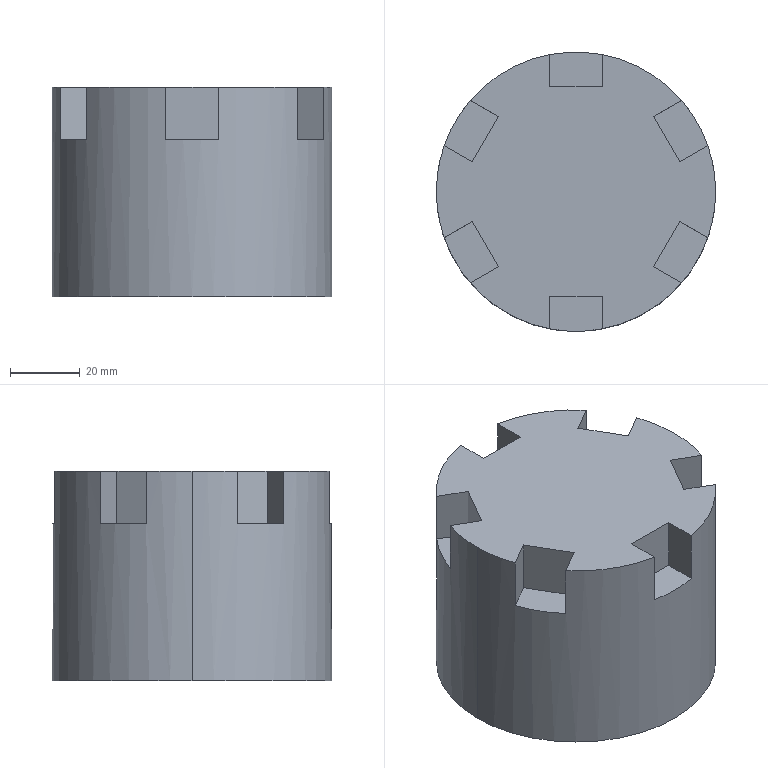Part | SolidWorks | features ICE 3, Extrusion 1 | 1 solid | 35 faces | box 80 x 80 x 60 mm | volume 237992 mm3 | plane 31 | cylinder 4 | commonest cylinder face diameters 39 x2 80 x2
STEP:
#1=CARTESIAN_POINT('',(40.,0.,60.));
#2=VERTEX_POINT('',#1);
#3=CARTESIAN_POINT('',(37.777,13.15,60.));
#4=VERTEX_POINT('',#3);
#5=CARTESIAN_POINT('',(0.,0.,60.));
#6=DIRECTION('',(0.,0.,1.));
#7=DIRECTION('',(1.,0.,0.));
#8=AXIS2_PLACEMENT_3D('',#5,#6,#7);
#9=CIRCLE('',#8,40.);
#10=EDGE_CURVE('',#2,#4,#9,.T.);
#11=ORIENTED_EDGE('',*,*,#10,.F.);
#12=CARTESIAN_POINT('',(40.,0.,0.));
#13=VERTEX_POINT('',#12);
#14=CARTESIAN_POINT('',(40.,0.,60.));
#15=DIRECTION('',(0.,0.,-1.));
#16=VECTOR('',#15,1000.);
#17=LINE('',#14,#16);
#18=EDGE_CURVE('',#2,#13,#17,.T.);
#19=ORIENTED_EDGE('',*,*,#18,.T.);
#20=CARTESIAN_POINT('',(-40.,0.,0.));
#21=VERTEX_POINT('',#20);
#22=CARTESIAN_POINT('',(0.,0.,0.));
#23=DIRECTION('',(0.,0.,1.));
#24=DIRECTION('',(1.,0.,0.));
#25=AXIS2_PLACEMENT_3D('',#22,#23,#24);
#26=CIRCLE('',#25,40.);
#27=EDGE_CURVE('',#13,#21,#26,.T.);
#28=ORIENTED_EDGE('',*,*,#27,.T.);
#29=CARTESIAN_POINT('',(-40.,0.,60.));
#30=VERTEX_POINT('',#29);
#31=CARTESIAN_POINT('',(-40.,0.,60.));
#32=DIRECTION('',(0.,0.,-1.));
#33=VECTOR('',#32,1000.);
#34=LINE('',#31,#33);
#35=EDGE_CURVE('',#30,#21,#34,.T.);
#36=ORIENTED_EDGE('',*,*,#35,.F.);
#37=CARTESIAN_POINT('',(-37.777,13.15,60.));
#38=VERTEX_POINT('',#37);
#39=CARTESIAN_POINT('',(0.,0.,60.));
#40=DIRECTION('',(0.,0.,1.));
#41=DIRECTION('',(1.,0.,0.));
#42=AXIS2_PLACEMENT_3D('',#39,#40,#41);
#43=CIRCLE('',#42,40.);
#44=EDGE_CURVE('',#38,#30,#43,.T.);
#45=ORIENTED_EDGE('',*,*,#44,.F.);
#46=CARTESIAN_POINT('',(-37.777,13.15,45.));
#47=VERTEX_POINT('',#46);
#48=CARTESIAN_POINT('',(-37.777,13.15,45.));
#49=DIRECTION('',(0.,0.,1.));
#50=VECTOR('',#49,1000.);
#51=LINE('',#48,#50);
#52=EDGE_CURVE('',#47,#38,#51,.T.);
#53=ORIENTED_EDGE('',*,*,#52,.F.);
#54=CARTESIAN_POINT('',(-30.277,26.14,45.));
#55=VERTEX_POINT('',#54);
#56=CARTESIAN_POINT('',(0.,0.,45.));
#57=DIRECTION('',(0.,0.,1.));
#58=DIRECTION('',(1.,0.,0.));
#59=AXIS2_PLACEMENT_3D('',#56,#57,#58);
#60=CIRCLE('',#59,40.);
#61=EDGE_CURVE('',#55,#47,#60,.T.);
#62=ORIENTED_EDGE('',*,*,#61,.F.);
#63=CARTESIAN_POINT('',(-30.277,26.14,60.));
#64=VERTEX_POINT('',#63);
#65=CARTESIAN_POINT('',(-30.277,26.14,45.));
#66=DIRECTION('',(0.,0.,1.));
#67=VECTOR('',#66,1000.);
#68=LINE('',#65,#67);
#69=EDGE_CURVE('',#55,#64,#68,.T.);
#70=ORIENTED_EDGE('',*,*,#69,.T.);
#71=CARTESIAN_POINT('',(-7.5,39.291,60.));
#72=VERTEX_POINT('',#71);
#73=CARTESIAN_POINT('',(0.,0.,60.));
#74=DIRECTION('',(0.,0.,1.));
#75=DIRECTION('',(1.,0.,0.));
#76=AXIS2_PLACEMENT_3D('',#73,#74,#75);
#77=CIRCLE('',#76,40.);
#78=EDGE_CURVE('',#72,#64,#77,.T.);
#79=ORIENTED_EDGE('',*,*,#78,.F.);
#80=CARTESIAN_POINT('',(-7.5,39.291,45.));
#81=VERTEX_POINT('',#80);
#82=CARTESIAN_POINT('',(-7.5,39.291,45.));
#83=DIRECTION('',(0.,0.,1.));
#84=VECTOR('',#83,1000.);
#85=LINE('',#82,#84);
#86=EDGE_CURVE('',#81,#72,#85,.T.);
#87=ORIENTED_EDGE('',*,*,#86,.F.);
#88=CARTESIAN_POINT('',(7.5,39.291,45.));
#89=VERTEX_POINT('',#88);
#90=CARTESIAN_POINT('',(0.,0.,45.));
#91=DIRECTION('',(0.,0.,1.));
#92=DIRECTION('',(1.,0.,0.));
#93=AXIS2_PLACEMENT_3D('',#90,#91,#92);
#94=CIRCLE('',#93,40.);
#95=EDGE_CURVE('',#89,#81,#94,.T.);
#96=ORIENTED_EDGE('',*,*,#95,.F.);
#97=CARTESIAN_POINT('',(7.5,39.291,60.));
#98=VERTEX_POINT('',#97);
#99=CARTESIAN_POINT('',(7.5,39.291,45.));
#100=DIRECTION('',(0.,0.,1.));
#101=VECTOR('',#100,1000.);
#102=LINE('',#99,#101);
#103=EDGE_CURVE('',#89,#98,#102,.T.);
#104=ORIENTED_EDGE('',*,*,#103,.T.);
#105=CARTESIAN_POINT('',(30.277,26.14,60.));
#106=VERTEX_POINT('',#105);
#107=CARTESIAN_POINT('',(0.,0.,60.));
#108=DIRECTION('',(0.,0.,1.));
#109=DIRECTION('',(1.,0.,0.));
#110=AXIS2_PLACEMENT_3D('',#107,#108,#109);
#111=CIRCLE('',#110,40.);
#112=EDGE_CURVE('',#106,#98,#111,.T.);
#113=ORIENTED_EDGE('',*,*,#112,.F.);
#114=CARTESIAN_POINT('',(30.277,26.14,45.));
#115=VERTEX_POINT('',#114);
#116=CARTESIAN_POINT('',(30.277,26.14,45.));
#117=DIRECTION('',(0.,0.,1.));
#118=VECTOR('',#117,1000.);
#119=LINE('',#116,#118);
#120=EDGE_CURVE('',#115,#106,#119,.T.);
#121=ORIENTED_EDGE('',*,*,#120,.F.);
#122=CARTESIAN_POINT('',(37.777,13.15,45.));
#123=VERTEX_POINT('',#122);
#124=CARTESIAN_POINT('',(0.,0.,45.));
#125=DIRECTION('',(0.,0.,1.));
#126=DIRECTION('',(1.,0.,0.));
#127=AXIS2_PLACEMENT_3D('',#124,#125,#126);
#128=CIRCLE('',#127,40.);
#129=EDGE_CURVE('',#123,#115,#128,.T.);
#130=ORIENTED_EDGE('',*,*,#129,.F.);
#131=CARTESIAN_POINT('',(37.777,13.15,45.));
#132=DIRECTION('',(0.,0.,1.));
#133=VECTOR('',#132,1000.);
#134=LINE('',#131,#133);
#135=EDGE_CURVE('',#123,#4,#134,.T.);
#136=ORIENTED_EDGE('',*,*,#135,.T.);
#137=EDGE_LOOP('',(#11,#19,#28,#36,#45,#53,#62,#70,#79,#87,#96,#104,#113,#121,#130,#136));
#138=FACE_OUTER_BOUND('',#137,.T.);
#139=CARTESIAN_POINT('',(0.,0.,60.));
#140=DIRECTION('',(0.,0.,-1.));
#141=DIRECTION('',(-1.,0.,0.));
#142=AXIS2_PLACEMENT_3D('',#139,#140,#141);
#143=CYLINDRICAL_SURFACE('',#142,40.);
#144=ADVANCED_FACE('',(#138),#143,.T.);
#145=CARTESIAN_POINT('',(-19.5,0.,40.));
#146=VERTEX_POINT('',#145);
#147=CARTESIAN_POINT('',(19.5,0.,40.));
#148=VERTEX_POINT('',#147);
#149=CARTESIAN_POINT('',(0.,0.,40.));
#150=DIRECTION('',(0.,0.,1.));
#151=DIRECTION('',(1.,0.,0.));
#152=AXIS2_PLACEMENT_3D('',#149,#150,#151);
#153=CIRCLE('',#152,19.5);
#154=EDGE_CURVE('',#146,#148,#153,.T.);
#155=ORIENTED_EDGE('',*,*,#154,.T.);
#156=CARTESIAN_POINT('',(19.5,0.,0.));
#157=VERTEX_POINT('',#156);
#158=CARTESIAN_POINT('',(19.5,0.,40.));
#159=DIRECTION('',(0.,0.,-1.));
#160=VECTOR('',#159,1000.);
#161=LINE('',#158,#160);
#162=EDGE_CURVE('',#148,#157,#161,.T.);
#163=ORIENTED_EDGE('',*,*,#162,.T.);
#164=CARTESIAN_POINT('',(-19.5,0.,0.));
#165=VERTEX_POINT('',#164);
#166=CARTESIAN_POINT('',(0.,0.,0.));
#167=DIRECTION('',(0.,0.,1.));
#168=DIRECTION('',(1.,0.,0.));
#169=AXIS2_PLACEMENT_3D('',#166,#167,#168);
#170=CIRCLE('',#169,19.5);
#171=EDGE_CURVE('',#165,#157,#170,.T.);
#172=ORIENTED_EDGE('',*,*,#171,.F.);
#173=CARTESIAN_POINT('',(-19.5,0.,40.));
#174=DIRECTION('',(0.,0.,-1.));
#175=VECTOR('',#174,1000.);
#176=LINE('',#173,#175);
#177=EDGE_CURVE('',#146,#165,#176,.T.);
#178=ORIENTED_EDGE('',*,*,#177,.F.);
#179=EDGE_LOOP('',(#155,#163,#172,#178));
#180=FACE_OUTER_BOUND('',#179,.T.);
#181=CARTESIAN_POINT('',(0.,0.,40.));
#182=DIRECTION('',(0.,0.,-1.));
#183=DIRECTION('',(-1.,0.,0.));
#184=AXIS2_PLACEMENT_3D('',#181,#182,#183);
#185=CYLINDRICAL_SURFACE('',#184,19.5);
#186=ADVANCED_FACE('',(#180),#185,.F.);
#187=CARTESIAN_POINT('',(0.,0.,0.));
#188=DIRECTION('',(0.,0.,1.));
#189=DIRECTION('',(1.,0.,0.));
#190=AXIS2_PLACEMENT_3D('',#187,#188,#189);
#191=CIRCLE('',#190,40.);
#192=EDGE_CURVE('',#21,#13,#191,.T.);
#193=ORIENTED_EDGE('',*,*,#192,.F.);
#194=ORIENTED_EDGE('',*,*,#27,.F.);
#195=EDGE_LOOP('',(#193,#194));
#196=FACE_OUTER_BOUND('',#195,.T.);
#197=CARTESIAN_POINT('',(-10.,23.,0.));
#198=VERTEX_POINT('',#197);
#199=CARTESIAN_POINT('',(-10.,16.741,0.));
#200=VERTEX_POINT('',#199);
#201=CARTESIAN_POINT('',(-10.,23.,0.));
#202=DIRECTION('',(0.,-1.,0.));
#203=VECTOR('',#202,1000.);
#204=LINE('',#201,#203);
#205=EDGE_CURVE('',#198,#200,#204,.T.);
#206=ORIENTED_EDGE('',*,*,#205,.T.);
#207=CARTESIAN_POINT('',(0.,0.,0.));
#208=DIRECTION('',(0.,0.,1.));
#209=DIRECTION('',(1.,0.,0.));
#210=AXIS2_PLACEMENT_3D('',#207,#208,#209);
#211=CIRCLE('',#210,19.5);
#212=EDGE_CURVE('',#200,#165,#211,.T.);
#213=ORIENTED_EDGE('',*,*,#212,.T.);
#214=ORIENTED_EDGE('',*,*,#171,.T.);
#215=CARTESIAN_POINT('',(10.,16.741,0.));
#216=VERTEX_POINT('',#215);
#217=CARTESIAN_POINT('',(0.,0.,0.));
#218=DIRECTION('',(0.,0.,1.));
#219=DIRECTION('',(1.,0.,0.));
#220=AXIS2_PLACEMENT_3D('',#217,#218,#219);
#221=CIRCLE('',#220,19.5);
#222=EDGE_CURVE('',#157,#216,#221,.T.);
#223=ORIENTED_EDGE('',*,*,#222,.T.);
#224=CARTESIAN_POINT('',(10.,23.,0.));
#225=VERTEX_POINT('',#224);
#226=CARTESIAN_POINT('',(10.,23.,0.));
#227=DIRECTION('',(0.,-1.,0.));
#228=VECTOR('',#227,1000.);
#229=LINE('',#226,#228);
#230=EDGE_CURVE('',#225,#216,#229,.T.);
#231=ORIENTED_EDGE('',*,*,#230,.F.);
#232=CARTESIAN_POINT('',(10.,23.,0.));
#233=DIRECTION('',(-1.,0.,0.));
#234=VECTOR('',#233,1000.);
#235=LINE('',#232,#234);
#236=EDGE_CURVE('',#225,#198,#235,.T.);
#237=ORIENTED_EDGE('',*,*,#236,.T.);
#238=EDGE_LOOP('',(#206,#213,#214,#223,#231,#237));
#239=FACE_BOUND('',#238,.T.);
#240=CARTESIAN_POINT('',(0.,0.,0.));
#241=DIRECTION('',(0.,0.,1.));
#242=DIRECTION('',(1.,0.,0.));
#243=AXIS2_PLACEMENT_3D('',#240,#241,#242);
#244=PLANE('',#243);
#245=ADVANCED_FACE('',(#196,#239),#244,.F.);
#246=ORIENTED_EDGE('',*,*,#162,.F.);
#247=CARTESIAN_POINT('',(0.,0.,40.));
#248=DIRECTION('',(0.,0.,1.));
#249=DIRECTION('',(1.,0.,0.));
#250=AXIS2_PLACEMENT_3D('',#247,#248,#249);
#251=CIRCLE('',#250,19.5);
#252=EDGE_CURVE('',#148,#146,#251,.T.);
#253=ORIENTED_EDGE('',*,*,#252,.T.);
#254=ORIENTED_EDGE('',*,*,#177,.T.);
#255=ORIENTED_EDGE('',*,*,#212,.F.);
#256=CARTESIAN_POINT('',(-10.,16.741,30.));
#257=VERTEX_POINT('',#256);
#258=CARTESIAN_POINT('',(-10.,16.741,40.));
#259=DIRECTION('',(0.,0.,1.));
#260=VECTOR('',#259,1000.);
#261=LINE('',#258,#260);
#262=EDGE_CURVE('',#200,#257,#261,.T.);
#263=ORIENTED_EDGE('',*,*,#262,.T.);
#264=CARTESIAN_POINT('',(10.,16.741,30.));
#265=VERTEX_POINT('',#264);
#266=CARTESIAN_POINT('',(0.,0.,30.));
#267=DIRECTION('',(0.,0.,1.));
#268=DIRECTION('',(1.,0.,0.));
#269=AXIS2_PLACEMENT_3D('',#266,#267,#268);
#270=CIRCLE('',#269,19.5);
#271=EDGE_CURVE('',#265,#257,#270,.T.);
#272=ORIENTED_EDGE('',*,*,#271,.F.);
#273=CARTESIAN_POINT('',(10.,16.741,40.));
#274=DIRECTION('',(0.,0.,1.));
#275=VECTOR('',#274,1000.);
#276=LINE('',#273,#275);
#277=EDGE_CURVE('',#216,#265,#276,.T.);
#278=ORIENTED_EDGE('',*,*,#277,.F.);
#279=ORIENTED_EDGE('',*,*,#222,.F.);
#280=EDGE_LOOP('',(#246,#253,#254,#255,#263,#272,#278,#279));
#281=FACE_OUTER_BOUND('',#280,.T.);
#282=CARTESIAN_POINT('',(0.,0.,40.));
#283=DIRECTION('',(0.,0.,-1.));
#284=DIRECTION('',(-1.,0.,0.));
#285=AXIS2_PLACEMENT_3D('',#282,#283,#284);
#286=CYLINDRICAL_SURFACE('',#285,19.5);
#287=ADVANCED_FACE('',(#281),#286,.F.);
#288=ORIENTED_EDGE('',*,*,#18,.F.);
#289=CARTESIAN_POINT('',(37.777,-13.15,60.));
#290=VERTEX_POINT('',#289);
#291=CARTESIAN_POINT('',(0.,0.,60.));
#292=DIRECTION('',(0.,0.,1.));
#293=DIRECTION('',(1.,0.,0.));
#294=AXIS2_PLACEMENT_3D('',#291,#292,#293);
#295=CIRCLE('',#294,40.);
#296=EDGE_CURVE('',#290,#2,#295,.T.);
#297=ORIENTED_EDGE('',*,*,#296,.F.);
#298=CARTESIAN_POINT('',(37.777,-13.15,45.));
#299=VERTEX_POINT('',#298);
#300=CARTESIAN_POINT('',(37.777,-13.15,45.));
#301=DIRECTION('',(0.,0.,1.));
#302=VECTOR('',#301,1000.);
#303=LINE('',#300,#302);
#304=EDGE_CURVE('',#299,#290,#303,.T.);
#305=ORIENTED_EDGE('',*,*,#304,.F.);
#306=CARTESIAN_POINT('',(30.277,-26.14,45.));
#307=VERTEX_POINT('',#306);
#308=CARTESIAN_POINT('',(0.,0.,45.));
#309=DIRECTION('',(0.,0.,1.));
#310=DIRECTION('',(1.,0.,0.));
#311=AXIS2_PLACEMENT_3D('',#308,#309,#310);
#312=CIRCLE('',#311,40.);
#313=EDGE_CURVE('',#307,#299,#312,.T.);
#314=ORIENTED_EDGE('',*,*,#313,.F.);
#315=CARTESIAN_POINT('',(30.277,-26.14,60.));
#316=VERTEX_POINT('',#315);
#317=CARTESIAN_POINT('',(30.277,-26.14,45.));
#318=DIRECTION('',(0.,0.,1.));
#319=VECTOR('',#318,1000.);
#320=LINE('',#317,#319);
#321=EDGE_CURVE('',#307,#316,#320,.T.);
#322=ORIENTED_EDGE('',*,*,#321,.T.);
#323=CARTESIAN_POINT('',(7.5,-39.291,60.));
#324=VERTEX_POINT('',#323);
#325=CARTESIAN_POINT('',(0.,0.,60.));
#326=DIRECTION('',(0.,0.,1.));
#327=DIRECTION('',(1.,0.,0.));
#328=AXIS2_PLACEMENT_3D('',#325,#326,#327);
#329=CIRCLE('',#328,40.);
#330=EDGE_CURVE('',#324,#316,#329,.T.);
#331=ORIENTED_EDGE('',*,*,#330,.F.);
#332=CARTESIAN_POINT('',(7.5,-39.291,45.));
#333=VERTEX_POINT('',#332);
#334=CARTESIAN_POINT('',(7.5,-39.291,45.));
#335=DIRECTION('',(0.,0.,1.));
#336=VECTOR('',#335,1000.);
#337=LINE('',#334,#336);
#338=EDGE_CURVE('',#333,#324,#337,.T.);
#339=ORIENTED_EDGE('',*,*,#338,.F.);
#340=CARTESIAN_POINT('',(-7.5,-39.291,45.));
#341=VERTEX_POINT('',#340);
#342=CARTESIAN_POINT('',(0.,0.,45.));
#343=DIRECTION('',(0.,0.,1.));
#344=DIRECTION('',(1.,0.,0.));
#345=AXIS2_PLACEMENT_3D('',#342,#343,#344);
#346=CIRCLE('',#345,40.);
#347=EDGE_CURVE('',#341,#333,#346,.T.);
#348=ORIENTED_EDGE('',*,*,#347,.F.);
#349=CARTESIAN_POINT('',(-7.5,-39.291,60.));
#350=VERTEX_POINT('',#349);
#351=CARTESIAN_POINT('',(-7.5,-39.291,45.));
#352=DIRECTION('',(0.,0.,1.));
#353=VECTOR('',#352,1000.);
#354=LINE('',#351,#353);
#355=EDGE_CURVE('',#341,#350,#354,.T.);
#356=ORIENTED_EDGE('',*,*,#355,.T.);
#357=CARTESIAN_POINT('',(-30.277,-26.14,60.));
#358=VERTEX_POINT('',#357);
#359=CARTESIAN_POINT('',(0.,0.,60.));
#360=DIRECTION('',(0.,0.,1.));
#361=DIRECTION('',(1.,0.,0.));
#362=AXIS2_PLACEMENT_3D('',#359,#360,#361);
#363=CIRCLE('',#362,40.);
#364=EDGE_CURVE('',#358,#350,#363,.T.);
#365=ORIENTED_EDGE('',*,*,#364,.F.);
#366=CARTESIAN_POINT('',(-30.277,-26.14,45.));
#367=VERTEX_POINT('',#366);
#368=CARTESIAN_POINT('',(-30.277,-26.14,45.));
#369=DIRECTION('',(0.,0.,1.));
#370=VECTOR('',#369,1000.);
#371=LINE('',#368,#370);
#372=EDGE_CURVE('',#367,#358,#371,.T.);
#373=ORIENTED_EDGE('',*,*,#372,.F.);
#374=CARTESIAN_POINT('',(-37.777,-13.15,45.));
#375=VERTEX_POINT('',#374);
#376=CARTESIAN_POINT('',(0.,0.,45.));
#377=DIRECTION('',(0.,0.,1.));
#378=DIRECTION('',(1.,0.,0.));
#379=AXIS2_PLACEMENT_3D('',#376,#377,#378);
#380=CIRCLE('',#379,40.);
#381=EDGE_CURVE('',#375,#367,#380,.T.);
#382=ORIENTED_EDGE('',*,*,#381,.F.);
#383=CARTESIAN_POINT('',(-37.777,-13.15,60.));
#384=VERTEX_POINT('',#383);
#385=CARTESIAN_POINT('',(-37.777,-13.15,45.));
#386=DIRECTION('',(0.,0.,1.));
#387=VECTOR('',#386,1000.);
#388=LINE('',#385,#387);
#389=EDGE_CURVE('',#375,#384,#388,.T.);
#390=ORIENTED_EDGE('',*,*,#389,.T.);
#391=CARTESIAN_POINT('',(0.,0.,60.));
#392=DIRECTION('',(0.,0.,1.));
#393=DIRECTION('',(1.,0.,0.));
#394=AXIS2_PLACEMENT_3D('',#391,#392,#393);
#395=CIRCLE('',#394,40.);
#396=EDGE_CURVE('',#30,#384,#395,.T.);
#397=ORIENTED_EDGE('',*,*,#396,.F.);
#398=ORIENTED_EDGE('',*,*,#35,.T.);
#399=ORIENTED_EDGE('',*,*,#192,.T.);
#400=EDGE_LOOP('',(#288,#297,#305,#314,#322,#331,#339,#348,#356,#365,#373,#382,#390,#397,#398,#399));
#401=FACE_OUTER_BOUND('',#400,.T.);
#402=CARTESIAN_POINT('',(0.,0.,60.));
#403=DIRECTION('',(0.,0.,-1.));
#404=DIRECTION('',(-1.,0.,0.));
#405=AXIS2_PLACEMENT_3D('',#402,#403,#404);
#406=CYLINDRICAL_SURFACE('',#405,40.);
#407=ADVANCED_FACE('',(#401),#406,.T.);
#408=CARTESIAN_POINT('',(7.5,30.,60.));
#409=VERTEX_POINT('',#408);
#410=CARTESIAN_POINT('',(7.5,39.291,60.));
#411=DIRECTION('',(0.,1.,0.));
#412=VECTOR('',#411,1000.);
#413=LINE('',#410,#412);
#414=EDGE_CURVE('',#409,#98,#413,.T.);
#415=ORIENTED_EDGE('',*,*,#414,.F.);
#416=CARTESIAN_POINT('',(-7.5,30.,60.));
#417=VERTEX_POINT('',#416);
#418=CARTESIAN_POINT('',(-7.5,30.,60.));
#419=DIRECTION('',(1.,0.,0.));
#420=VECTOR('',#419,1000.);
#421=LINE('',#418,#420);
#422=EDGE_CURVE('',#417,#409,#421,.T.);
#423=ORIENTED_EDGE('',*,*,#422,.F.);
#424=CARTESIAN_POINT('',(-7.5,39.291,60.));
#425=DIRECTION('',(0.,-1.,0.));
#426=VECTOR('',#425,1000.);
#427=LINE('',#424,#426);
#428=EDGE_CURVE('',#72,#417,#427,.T.);
#429=ORIENTED_EDGE('',*,*,#428,.F.);
#430=ORIENTED_EDGE('',*,*,#78,.T.);
#431=CARTESIAN_POINT('',(-22.231,21.495,60.));
#432=VERTEX_POINT('',#431);
#433=CARTESIAN_POINT('',(-30.277,26.14,60.));
#434=DIRECTION('',(-0.866,0.5,0.));
#435=VECTOR('',#434,1000.);
#436=LINE('',#433,#435);
#437=EDGE_CURVE('',#432,#64,#436,.T.);
#438=ORIENTED_EDGE('',*,*,#437,.F.);
#439=CARTESIAN_POINT('',(-29.731,8.505,60.));
#440=VERTEX_POINT('',#439);
#441=CARTESIAN_POINT('',(-29.731,8.505,60.));
#442=DIRECTION('',(0.5,0.866,0.));
#443=VECTOR('',#442,1000.);
#444=LINE('',#441,#443);
#445=EDGE_CURVE('',#440,#432,#444,.T.);
#446=ORIENTED_EDGE('',*,*,#445,.F.);
#447=CARTESIAN_POINT('',(-37.777,13.15,60.));
#448=DIRECTION('',(0.866,-0.5,0.));
#449=VECTOR('',#448,1000.);
#450=LINE('',#447,#449);
#451=EDGE_CURVE('',#38,#440,#450,.T.);
#452=ORIENTED_EDGE('',*,*,#451,.F.);
#453=ORIENTED_EDGE('',*,*,#44,.T.);
#454=ORIENTED_EDGE('',*,*,#396,.T.);
#455=CARTESIAN_POINT('',(-29.731,-8.505,60.));
#456=VERTEX_POINT('',#455);
#457=CARTESIAN_POINT('',(-37.777,-13.15,60.));
#458=DIRECTION('',(-0.866,-0.5,0.));
#459=VECTOR('',#458,1000.);
#460=LINE('',#457,#459);
#461=EDGE_CURVE('',#456,#384,#460,.T.);
#462=ORIENTED_EDGE('',*,*,#461,.F.);
#463=CARTESIAN_POINT('',(-22.231,-21.495,60.));
#464=VERTEX_POINT('',#463);
#465=CARTESIAN_POINT('',(-22.231,-21.495,60.));
#466=DIRECTION('',(-0.5,0.866,0.));
#467=VECTOR('',#466,1000.);
#468=LINE('',#465,#467);
#469=EDGE_CURVE('',#464,#456,#468,.T.);
#470=ORIENTED_EDGE('',*,*,#469,.F.);
#471=CARTESIAN_POINT('',(-30.277,-26.14,60.));
#472=DIRECTION('',(0.866,0.5,0.));
#473=VECTOR('',#472,1000.);
#474=LINE('',#471,#473);
#475=EDGE_CURVE('',#358,#464,#474,.T.);
#476=ORIENTED_EDGE('',*,*,#475,.F.);
#477=ORIENTED_EDGE('',*,*,#364,.T.);
#478=CARTESIAN_POINT('',(-7.5,-30.,60.));
#479=VERTEX_POINT('',#478);
#480=CARTESIAN_POINT('',(-7.5,-39.291,60.));
#481=DIRECTION('',(0.,-1.,0.));
#482=VECTOR('',#481,1000.);
#483=LINE('',#480,#482);
#484=EDGE_CURVE('',#479,#350,#483,.T.);
#485=ORIENTED_EDGE('',*,*,#484,.F.);
#486=CARTESIAN_POINT('',(7.5,-30.,60.));
#487=VERTEX_POINT('',#486);
#488=CARTESIAN_POINT('',(7.5,-30.,60.));
#489=DIRECTION('',(-1.,0.,0.));
#490=VECTOR('',#489,1000.);
#491=LINE('',#488,#490);
#492=EDGE_CURVE('',#487,#479,#491,.T.);
#493=ORIENTED_EDGE('',*,*,#492,.F.);
#494=CARTESIAN_POINT('',(7.5,-39.291,60.));
#495=DIRECTION('',(0.,1.,0.));
#496=VECTOR('',#495,1000.);
#497=LINE('',#494,#496);
#498=EDGE_CURVE('',#324,#487,#497,.T.);
#499=ORIENTED_EDGE('',*,*,#498,.F.);
#500=ORIENTED_EDGE('',*,*,#330,.T.);
#501=CARTESIAN_POINT('',(22.231,-21.495,60.));
#502=VERTEX_POINT('',#501);
#503=CARTESIAN_POINT('',(30.277,-26.14,60.));
#504=DIRECTION('',(0.866,-0.5,0.));
#505=VECTOR('',#504,1000.);
#506=LINE('',#503,#505);
#507=EDGE_CURVE('',#502,#316,#506,.T.);
#508=ORIENTED_EDGE('',*,*,#507,.F.);
#509=CARTESIAN_POINT('',(29.731,-8.505,60.));
#510=VERTEX_POINT('',#509);
#511=CARTESIAN_POINT('',(29.731,-8.505,60.));
#512=DIRECTION('',(-0.5,-0.866,0.));
#513=VECTOR('',#512,1000.);
#514=LINE('',#511,#513);
#515=EDGE_CURVE('',#510,#502,#514,.T.);
#516=ORIENTED_EDGE('',*,*,#515,.F.);
#517=CARTESIAN_POINT('',(37.777,-13.15,60.));
#518=DIRECTION('',(-0.866,0.5,0.));
#519=VECTOR('',#518,1000.);
#520=LINE('',#517,#519);
#521=EDGE_CURVE('',#290,#510,#520,.T.);
#522=ORIENTED_EDGE('',*,*,#521,.F.);
#523=ORIENTED_EDGE('',*,*,#296,.T.);
#524=ORIENTED_EDGE('',*,*,#10,.T.);
#525=CARTESIAN_POINT('',(29.731,8.505,60.));
#526=VERTEX_POINT('',#525);
#527=CARTESIAN_POINT('',(37.777,13.15,60.));
#528=DIRECTION('',(0.866,0.5,0.));
#529=VECTOR('',#528,1000.);
#530=LINE('',#527,#529);
#531=EDGE_CURVE('',#526,#4,#530,.T.);
#532=ORIENTED_EDGE('',*,*,#531,.F.);
#533=CARTESIAN_POINT('',(22.231,21.495,60.));
#534=VERTEX_POINT('',#533);
#535=CARTESIAN_POINT('',(22.231,21.495,60.));
#536=DIRECTION('',(0.5,-0.866,0.));
#537=VECTOR('',#536,1000.);
#538=LINE('',#535,#537);
#539=EDGE_CURVE('',#534,#526,#538,.T.);
#540=ORIENTED_EDGE('',*,*,#539,.F.);
#541=CARTESIAN_POINT('',(30.277,26.14,60.));
#542=DIRECTION('',(-0.866,-0.5,0.));
#543=VECTOR('',#542,1000.);
#544=LINE('',#541,#543);
#545=EDGE_CURVE('',#106,#534,#544,.T.);
#546=ORIENTED_EDGE('',*,*,#545,.F.);
#547=ORIENTED_EDGE('',*,*,#112,.T.);
#548=EDGE_LOOP('',(#415,#423,#429,#430,#438,#446,#452,#453,#454,#462,#470,#476,#477,#485,#493,#499,#500,#508,#516,#522,#523,#524,#532,#540,#546,#547));
#549=FACE_OUTER_BOUND('',#548,.T.);
#550=CARTESIAN_POINT('',(0.,0.,60.));
#551=DIRECTION('',(0.,0.,1.));
#552=DIRECTION('',(1.,0.,0.));
#553=AXIS2_PLACEMENT_3D('',#550,#551,#552);
#554=PLANE('',#553);
#555=ADVANCED_FACE('',(#549),#554,.T.);
#556=ORIENTED_EDGE('',*,*,#154,.F.);
#557=ORIENTED_EDGE('',*,*,#252,.F.);
#558=EDGE_LOOP('',(#556,#557));
#559=FACE_OUTER_BOUND('',#558,.T.);
#560=CARTESIAN_POINT('',(0.,0.,40.));
#561=DIRECTION('',(0.,0.,1.));
#562=DIRECTION('',(1.,0.,0.));
#563=AXIS2_PLACEMENT_3D('',#560,#561,#562);
#564=PLANE('',#563);
#565=ADVANCED_FACE('',(#559),#564,.F.);
#566=ORIENTED_EDGE('',*,*,#531,.T.);
#567=ORIENTED_EDGE('',*,*,#135,.F.);
#568=CARTESIAN_POINT('',(29.731,8.505,45.));
#569=VERTEX_POINT('',#568);
#570=CARTESIAN_POINT('',(37.777,13.15,45.));
#571=DIRECTION('',(0.866,0.5,0.));
#572=VECTOR('',#571,1000.);
#573=LINE('',#570,#572);
#574=EDGE_CURVE('',#569,#123,#573,.T.);
#575=ORIENTED_EDGE('',*,*,#574,.F.);
#576=CARTESIAN_POINT('',(29.731,8.505,45.));
#577=DIRECTION('',(0.,0.,1.));
#578=VECTOR('',#577,1000.);
#579=LINE('',#576,#578);
#580=EDGE_CURVE('',#569,#526,#579,.T.);
#581=ORIENTED_EDGE('',*,*,#580,.T.);
#582=EDGE_LOOP('',(#566,#567,#575,#581));
#583=FACE_OUTER_BOUND('',#582,.T.);
#584=CARTESIAN_POINT('',(37.777,13.15,45.));
#585=DIRECTION('',(0.5,-0.866,0.));
#586=DIRECTION('',(0.866,0.5,0.));
#587=AXIS2_PLACEMENT_3D('',#584,#585,#586);
#588=PLANE('',#587);
#589=ADVANCED_FACE('',(#583),#588,.F.);
#590=ORIENTED_EDGE('',*,*,#539,.T.);
#591=ORIENTED_EDGE('',*,*,#580,.F.);
#592=CARTESIAN_POINT('',(22.231,21.495,45.));
#593=VERTEX_POINT('',#592);
#594=CARTESIAN_POINT('',(22.231,21.495,45.));
#595=DIRECTION('',(0.5,-0.866,0.));
#596=VECTOR('',#595,1000.);
#597=LINE('',#594,#596);
#598=EDGE_CURVE('',#593,#569,#597,.T.);
#599=ORIENTED_EDGE('',*,*,#598,.F.);
#600=CARTESIAN_POINT('',(22.231,21.495,45.));
#601=DIRECTION('',(0.,0.,1.));
#602=VECTOR('',#601,1000.);
#603=LINE('',#600,#602);
#604=EDGE_CURVE('',#593,#534,#603,.T.);
#605=ORIENTED_EDGE('',*,*,#604,.T.);
#606=EDGE_LOOP('',(#590,#591,#599,#605));
#607=FACE_OUTER_BOUND('',#606,.T.);
#608=CARTESIAN_POINT('',(22.231,21.495,45.));
#609=DIRECTION('',(-0.866,-0.5,0.));
#610=DIRECTION('',(0.5,-0.866,0.));
#611=AXIS2_PLACEMENT_3D('',#608,#609,#610);
#612=PLANE('',#611);
#613=ADVANCED_FACE('',(#607),#612,.F.);
#614=ORIENTED_EDGE('',*,*,#545,.T.);
#615=ORIENTED_EDGE('',*,*,#604,.F.);
#616=CARTESIAN_POINT('',(30.277,26.14,45.));
#617=DIRECTION('',(-0.866,-0.5,0.));
#618=VECTOR('',#617,1000.);
#619=LINE('',#616,#618);
#620=EDGE_CURVE('',#115,#593,#619,.T.);
#621=ORIENTED_EDGE('',*,*,#620,.F.);
#622=ORIENTED_EDGE('',*,*,#120,.T.);
#623=EDGE_LOOP('',(#614,#615,#621,#622));
#624=FACE_OUTER_BOUND('',#623,.T.);
#625=CARTESIAN_POINT('',(30.277,26.14,45.));
#626=DIRECTION('',(-0.5,0.866,0.));
#627=DIRECTION('',(-0.866,-0.5,0.));
#628=AXIS2_PLACEMENT_3D('',#625,#626,#627);
#629=PLANE('',#628);
#630=ADVANCED_FACE('',(#624),#629,.F.);
#631=ORIENTED_EDGE('',*,*,#129,.T.);
#632=ORIENTED_EDGE('',*,*,#620,.T.);
#633=ORIENTED_EDGE('',*,*,#598,.T.);
#634=ORIENTED_EDGE('',*,*,#574,.T.);
#635=EDGE_LOOP('',(#631,#632,#633,#634));
#636=FACE_OUTER_BOUND('',#635,.T.);
#637=CARTESIAN_POINT('',(0.,0.,45.));
#638=DIRECTION('',(0.,0.,1.));
#639=DIRECTION('',(1.,0.,0.));
#640=AXIS2_PLACEMENT_3D('',#637,#638,#639);
#641=PLANE('',#640);
#642=ADVANCED_FACE('',(#636),#641,.T.);
#643=ORIENTED_EDGE('',*,*,#507,.T.);
#644=ORIENTED_EDGE('',*,*,#321,.F.);
#645=CARTESIAN_POINT('',(22.231,-21.495,45.));
#646=VERTEX_POINT('',#645);
#647=CARTESIAN_POINT('',(30.277,-26.14,45.));
#648=DIRECTION('',(0.866,-0.5,0.));
#649=VECTOR('',#648,1000.);
#650=LINE('',#647,#649);
#651=EDGE_CURVE('',#646,#307,#650,.T.);
#652=ORIENTED_EDGE('',*,*,#651,.F.);
#653=CARTESIAN_POINT('',(22.231,-21.495,45.));
#654=DIRECTION('',(0.,0.,1.));
#655=VECTOR('',#654,1000.);
#656=LINE('',#653,#655);
#657=EDGE_CURVE('',#646,#502,#656,.T.);
#658=ORIENTED_EDGE('',*,*,#657,.T.);
#659=EDGE_LOOP('',(#643,#644,#652,#658));
#660=FACE_OUTER_BOUND('',#659,.T.);
#661=CARTESIAN_POINT('',(30.277,-26.14,45.));
#662=DIRECTION('',(-0.5,-0.866,0.));
#663=DIRECTION('',(0.866,-0.5,0.));
#664=AXIS2_PLACEMENT_3D('',#661,#662,#663);
#665=PLANE('',#664);
#666=ADVANCED_FACE('',(#660),#665,.F.);
#667=ORIENTED_EDGE('',*,*,#515,.T.);
#668=ORIENTED_EDGE('',*,*,#657,.F.);
#669=CARTESIAN_POINT('',(29.731,-8.505,45.));
#670=VERTEX_POINT('',#669);
#671=CARTESIAN_POINT('',(29.731,-8.505,45.));
#672=DIRECTION('',(-0.5,-0.866,0.));
#673=VECTOR('',#672,1000.);
#674=LINE('',#671,#673);
#675=EDGE_CURVE('',#670,#646,#674,.T.);
#676=ORIENTED_EDGE('',*,*,#675,.F.);
#677=CARTESIAN_POINT('',(29.731,-8.505,45.));
#678=DIRECTION('',(0.,0.,1.));
#679=VECTOR('',#678,1000.);
#680=LINE('',#677,#679);
#681=EDGE_CURVE('',#670,#510,#680,.T.);
#682=ORIENTED_EDGE('',*,*,#681,.T.);
#683=EDGE_LOOP('',(#667,#668,#676,#682));
#684=FACE_OUTER_BOUND('',#683,.T.);
#685=CARTESIAN_POINT('',(29.731,-8.505,45.));
#686=DIRECTION('',(-0.866,0.5,0.));
#687=DIRECTION('',(-0.5,-0.866,0.));
#688=AXIS2_PLACEMENT_3D('',#685,#686,#687);
#689=PLANE('',#688);
#690=ADVANCED_FACE('',(#684),#689,.F.);
#691=ORIENTED_EDGE('',*,*,#521,.T.);
#692=ORIENTED_EDGE('',*,*,#681,.F.);
#693=CARTESIAN_POINT('',(37.777,-13.15,45.));
#694=DIRECTION('',(-0.866,0.5,0.));
#695=VECTOR('',#694,1000.);
#696=LINE('',#693,#695);
#697=EDGE_CURVE('',#299,#670,#696,.T.);
#698=ORIENTED_EDGE('',*,*,#697,.F.);
#699=ORIENTED_EDGE('',*,*,#304,.T.);
#700=EDGE_LOOP('',(#691,#692,#698,#699));
#701=FACE_OUTER_BOUND('',#700,.T.);
#702=CARTESIAN_POINT('',(37.777,-13.15,45.));
#703=DIRECTION('',(0.5,0.866,0.));
#704=DIRECTION('',(-0.866,0.5,0.));
#705=AXIS2_PLACEMENT_3D('',#702,#703,#704);
#706=PLANE('',#705);
#707=ADVANCED_FACE('',(#701),#706,.F.);
#708=ORIENTED_EDGE('',*,*,#313,.T.);
#709=ORIENTED_EDGE('',*,*,#697,.T.);
#710=ORIENTED_EDGE('',*,*,#675,.T.);
#711=ORIENTED_EDGE('',*,*,#651,.T.);
#712=EDGE_LOOP('',(#708,#709,#710,#711));
#713=FACE_OUTER_BOUND('',#712,.T.);
#714=CARTESIAN_POINT('',(0.,0.,45.));
#715=DIRECTION('',(0.,0.,1.));
#716=DIRECTION('',(1.,0.,0.));
#717=AXIS2_PLACEMENT_3D('',#714,#715,#716);
#718=PLANE('',#717);
#719=ADVANCED_FACE('',(#713),#718,.T.);
#720=ORIENTED_EDGE('',*,*,#484,.T.);
#721=ORIENTED_EDGE('',*,*,#355,.F.);
#722=CARTESIAN_POINT('',(-7.5,-30.,45.));
#723=VERTEX_POINT('',#722);
#724=CARTESIAN_POINT('',(-7.5,-39.291,45.));
#725=DIRECTION('',(0.,-1.,0.));
#726=VECTOR('',#725,1000.);
#727=LINE('',#724,#726);
#728=EDGE_CURVE('',#723,#341,#727,.T.);
#729=ORIENTED_EDGE('',*,*,#728,.F.);
#730=CARTESIAN_POINT('',(-7.5,-30.,45.));
#731=DIRECTION('',(0.,0.,1.));
#732=VECTOR('',#731,1000.);
#733=LINE('',#730,#732);
#734=EDGE_CURVE('',#723,#479,#733,.T.);
#735=ORIENTED_EDGE('',*,*,#734,.T.);
#736=EDGE_LOOP('',(#720,#721,#729,#735));
#737=FACE_OUTER_BOUND('',#736,.T.);
#738=CARTESIAN_POINT('',(-7.5,-39.291,45.));
#739=DIRECTION('',(-1.,0.,0.));
#740=DIRECTION('',(0.,-1.,0.));
#741=AXIS2_PLACEMENT_3D('',#738,#739,#740);
#742=PLANE('',#741);
#743=ADVANCED_FACE('',(#737),#742,.F.);
#744=ORIENTED_EDGE('',*,*,#492,.T.);
#745=ORIENTED_EDGE('',*,*,#734,.F.);
#746=CARTESIAN_POINT('',(7.5,-30.,45.));
#747=VERTEX_POINT('',#746);
#748=CARTESIAN_POINT('',(7.5,-30.,45.));
#749=DIRECTION('',(-1.,0.,0.));
#750=VECTOR('',#749,1000.);
#751=LINE('',#748,#750);
#752=EDGE_CURVE('',#747,#723,#751,.T.);
#753=ORIENTED_EDGE('',*,*,#752,.F.);
#754=CARTESIAN_POINT('',(7.5,-30.,45.));
#755=DIRECTION('',(0.,0.,1.));
#756=VECTOR('',#755,1000.);
#757=LINE('',#754,#756);
#758=EDGE_CURVE('',#747,#487,#757,.T.);
#759=ORIENTED_EDGE('',*,*,#758,.T.);
#760=EDGE_LOOP('',(#744,#745,#753,#759));
#761=FACE_OUTER_BOUND('',#760,.T.);
#762=CARTESIAN_POINT('',(7.5,-30.,45.));
#763=DIRECTION('',(0.,1.,0.));
#764=DIRECTION('',(-1.,0.,0.));
#765=AXIS2_PLACEMENT_3D('',#762,#763,#764);
#766=PLANE('',#765);
#767=ADVANCED_FACE('',(#761),#766,.F.);
#768=ORIENTED_EDGE('',*,*,#498,.T.);
#769=ORIENTED_EDGE('',*,*,#758,.F.);
#770=CARTESIAN_POINT('',(7.5,-39.291,45.));
#771=DIRECTION('',(0.,1.,0.));
#772=VECTOR('',#771,1000.);
#773=LINE('',#770,#772);
#774=EDGE_CURVE('',#333,#747,#773,.T.);
#775=ORIENTED_EDGE('',*,*,#774,.F.);
#776=ORIENTED_EDGE('',*,*,#338,.T.);
#777=EDGE_LOOP('',(#768,#769,#775,#776));
#778=FACE_OUTER_BOUND('',#777,.T.);
#779=CARTESIAN_POINT('',(7.5,-39.291,45.));
#780=DIRECTION('',(1.,0.,0.));
#781=DIRECTION('',(0.,1.,0.));
#782=AXIS2_PLACEMENT_3D('',#779,#780,#781);
#783=PLANE('',#782);
#784=ADVANCED_FACE('',(#778),#783,.F.);
#785=ORIENTED_EDGE('',*,*,#347,.T.);
#786=ORIENTED_EDGE('',*,*,#774,.T.);
#787=ORIENTED_EDGE('',*,*,#752,.T.);
#788=ORIENTED_EDGE('',*,*,#728,.T.);
#789=EDGE_LOOP('',(#785,#786,#787,#788));
#790=FACE_OUTER_BOUND('',#789,.T.);
#791=CARTESIAN_POINT('',(0.,0.,45.));
#792=DIRECTION('',(0.,0.,1.));
#793=DIRECTION('',(1.,0.,0.));
#794=AXIS2_PLACEMENT_3D('',#791,#792,#793);
#795=PLANE('',#794);
#796=ADVANCED_FACE('',(#790),#795,.T.);
#797=ORIENTED_EDGE('',*,*,#461,.T.);
#798=ORIENTED_EDGE('',*,*,#389,.F.);
#799=CARTESIAN_POINT('',(-29.731,-8.505,45.));
#800=VERTEX_POINT('',#799);
#801=CARTESIAN_POINT('',(-37.777,-13.15,45.));
#802=DIRECTION('',(-0.866,-0.5,0.));
#803=VECTOR('',#802,1000.);
#804=LINE('',#801,#803);
#805=EDGE_CURVE('',#800,#375,#804,.T.);
#806=ORIENTED_EDGE('',*,*,#805,.F.);
#807=CARTESIAN_POINT('',(-29.731,-8.505,45.));
#808=DIRECTION('',(0.,0.,1.));
#809=VECTOR('',#808,1000.);
#810=LINE('',#807,#809);
#811=EDGE_CURVE('',#800,#456,#810,.T.);
#812=ORIENTED_EDGE('',*,*,#811,.T.);
#813=EDGE_LOOP('',(#797,#798,#806,#812));
#814=FACE_OUTER_BOUND('',#813,.T.);
#815=CARTESIAN_POINT('',(-37.777,-13.15,45.));
#816=DIRECTION('',(-0.5,0.866,0.));
#817=DIRECTION('',(-0.866,-0.5,0.));
#818=AXIS2_PLACEMENT_3D('',#815,#816,#817);
#819=PLANE('',#818);
#820=ADVANCED_FACE('',(#814),#819,.F.);
#821=ORIENTED_EDGE('',*,*,#469,.T.);
#822=ORIENTED_EDGE('',*,*,#811,.F.);
#823=CARTESIAN_POINT('',(-22.231,-21.495,45.));
#824=VERTEX_POINT('',#823);
#825=CARTESIAN_POINT('',(-22.231,-21.495,45.));
#826=DIRECTION('',(-0.5,0.866,0.));
#827=VECTOR('',#826,1000.);
#828=LINE('',#825,#827);
#829=EDGE_CURVE('',#824,#800,#828,.T.);
#830=ORIENTED_EDGE('',*,*,#829,.F.);
#831=CARTESIAN_POINT('',(-22.231,-21.495,45.));
#832=DIRECTION('',(0.,0.,1.));
#833=VECTOR('',#832,1000.);
#834=LINE('',#831,#833);
#835=EDGE_CURVE('',#824,#464,#834,.T.);
#836=ORIENTED_EDGE('',*,*,#835,.T.);
#837=EDGE_LOOP('',(#821,#822,#830,#836));
#838=FACE_OUTER_BOUND('',#837,.T.);
#839=CARTESIAN_POINT('',(-22.231,-21.495,45.));
#840=DIRECTION('',(0.866,0.5,0.));
#841=DIRECTION('',(-0.5,0.866,0.));
#842=AXIS2_PLACEMENT_3D('',#839,#840,#841);
#843=PLANE('',#842);
#844=ADVANCED_FACE('',(#838),#843,.F.);
#845=ORIENTED_EDGE('',*,*,#475,.T.);
#846=ORIENTED_EDGE('',*,*,#835,.F.);
#847=CARTESIAN_POINT('',(-30.277,-26.14,45.));
#848=DIRECTION('',(0.866,0.5,0.));
#849=VECTOR('',#848,1000.);
#850=LINE('',#847,#849);
#851=EDGE_CURVE('',#367,#824,#850,.T.);
#852=ORIENTED_EDGE('',*,*,#851,.F.);
#853=ORIENTED_EDGE('',*,*,#372,.T.);
#854=EDGE_LOOP('',(#845,#846,#852,#853));
#855=FACE_OUTER_BOUND('',#854,.T.);
#856=CARTESIAN_POINT('',(-30.277,-26.14,45.));
#857=DIRECTION('',(0.5,-0.866,0.));
#858=DIRECTION('',(0.866,0.5,0.));
#859=AXIS2_PLACEMENT_3D('',#856,#857,#858);
#860=PLANE('',#859);
#861=ADVANCED_FACE('',(#855),#860,.F.);
#862=ORIENTED_EDGE('',*,*,#381,.T.);
#863=ORIENTED_EDGE('',*,*,#851,.T.);
#864=ORIENTED_EDGE('',*,*,#829,.T.);
#865=ORIENTED_EDGE('',*,*,#805,.T.);
#866=EDGE_LOOP('',(#862,#863,#864,#865));
#867=FACE_OUTER_BOUND('',#866,.T.);
#868=CARTESIAN_POINT('',(0.,0.,45.));
#869=DIRECTION('',(0.,0.,1.));
#870=DIRECTION('',(1.,0.,0.));
#871=AXIS2_PLACEMENT_3D('',#868,#869,#870);
#872=PLANE('',#871);
#873=ADVANCED_FACE('',(#867),#872,.T.);
#874=ORIENTED_EDGE('',*,*,#437,.T.);
#875=ORIENTED_EDGE('',*,*,#69,.F.);
#876=CARTESIAN_POINT('',(-22.231,21.495,45.));
#877=VERTEX_POINT('',#876);
#878=CARTESIAN_POINT('',(-30.277,26.14,45.));
#879=DIRECTION('',(-0.866,0.5,0.));
#880=VECTOR('',#879,1000.);
#881=LINE('',#878,#880);
#882=EDGE_CURVE('',#877,#55,#881,.T.);
#883=ORIENTED_EDGE('',*,*,#882,.F.);
#884=CARTESIAN_POINT('',(-22.231,21.495,45.));
#885=DIRECTION('',(0.,0.,1.));
#886=VECTOR('',#885,1000.);
#887=LINE('',#884,#886);
#888=EDGE_CURVE('',#877,#432,#887,.T.);
#889=ORIENTED_EDGE('',*,*,#888,.T.);
#890=EDGE_LOOP('',(#874,#875,#883,#889));
#891=FACE_OUTER_BOUND('',#890,.T.);
#892=CARTESIAN_POINT('',(-30.277,26.14,45.));
#893=DIRECTION('',(0.5,0.866,0.));
#894=DIRECTION('',(-0.866,0.5,0.));
#895=AXIS2_PLACEMENT_3D('',#892,#893,#894);
#896=PLANE('',#895);
#897=ADVANCED_FACE('',(#891),#896,.F.);
#898=ORIENTED_EDGE('',*,*,#445,.T.);
#899=ORIENTED_EDGE('',*,*,#888,.F.);
#900=CARTESIAN_POINT('',(-29.731,8.505,45.));
#901=VERTEX_POINT('',#900);
#902=CARTESIAN_POINT('',(-29.731,8.505,45.));
#903=DIRECTION('',(0.5,0.866,0.));
#904=VECTOR('',#903,1000.);
#905=LINE('',#902,#904);
#906=EDGE_CURVE('',#901,#877,#905,.T.);
#907=ORIENTED_EDGE('',*,*,#906,.F.);
#908=CARTESIAN_POINT('',(-29.731,8.505,45.));
#909=DIRECTION('',(0.,0.,1.));
#910=VECTOR('',#909,1000.);
#911=LINE('',#908,#910);
#912=EDGE_CURVE('',#901,#440,#911,.T.);
#913=ORIENTED_EDGE('',*,*,#912,.T.);
#914=EDGE_LOOP('',(#898,#899,#907,#913));
#915=FACE_OUTER_BOUND('',#914,.T.);
#916=CARTESIAN_POINT('',(-29.731,8.505,45.));
#917=DIRECTION('',(0.866,-0.5,0.));
#918=DIRECTION('',(0.5,0.866,0.));
#919=AXIS2_PLACEMENT_3D('',#916,#917,#918);
#920=PLANE('',#919);
#921=ADVANCED_FACE('',(#915),#920,.F.);
#922=ORIENTED_EDGE('',*,*,#451,.T.);
#923=ORIENTED_EDGE('',*,*,#912,.F.);
#924=CARTESIAN_POINT('',(-37.777,13.15,45.));
#925=DIRECTION('',(0.866,-0.5,0.));
#926=VECTOR('',#925,1000.);
#927=LINE('',#924,#926);
#928=EDGE_CURVE('',#47,#901,#927,.T.);
#929=ORIENTED_EDGE('',*,*,#928,.F.);
#930=ORIENTED_EDGE('',*,*,#52,.T.);
#931=EDGE_LOOP('',(#922,#923,#929,#930));
#932=FACE_OUTER_BOUND('',#931,.T.);
#933=CARTESIAN_POINT('',(-37.777,13.15,45.));
#934=DIRECTION('',(-0.5,-0.866,0.));
#935=DIRECTION('',(0.866,-0.5,0.));
#936=AXIS2_PLACEMENT_3D('',#933,#934,#935);
#937=PLANE('',#936);
#938=ADVANCED_FACE('',(#932),#937,.F.);
#939=ORIENTED_EDGE('',*,*,#61,.T.);
#940=ORIENTED_EDGE('',*,*,#928,.T.);
#941=ORIENTED_EDGE('',*,*,#906,.T.);
#942=ORIENTED_EDGE('',*,*,#882,.T.);
#943=EDGE_LOOP('',(#939,#940,#941,#942));
#944=FACE_OUTER_BOUND('',#943,.T.);
#945=CARTESIAN_POINT('',(0.,0.,45.));
#946=DIRECTION('',(0.,0.,1.));
#947=DIRECTION('',(1.,0.,0.));
#948=AXIS2_PLACEMENT_3D('',#945,#946,#947);
#949=PLANE('',#948);
#950=ADVANCED_FACE('',(#944),#949,.T.);
#951=ORIENTED_EDGE('',*,*,#414,.T.);
#952=ORIENTED_EDGE('',*,*,#103,.F.);
#953=CARTESIAN_POINT('',(7.5,30.,45.));
#954=VERTEX_POINT('',#953);
#955=CARTESIAN_POINT('',(7.5,39.291,45.));
#956=DIRECTION('',(0.,1.,0.));
#957=VECTOR('',#956,1000.);
#958=LINE('',#955,#957);
#959=EDGE_CURVE('',#954,#89,#958,.T.);
#960=ORIENTED_EDGE('',*,*,#959,.F.);
#961=CARTESIAN_POINT('',(7.5,30.,45.));
#962=DIRECTION('',(0.,0.,1.));
#963=VECTOR('',#962,1000.);
#964=LINE('',#961,#963);
#965=EDGE_CURVE('',#954,#409,#964,.T.);
#966=ORIENTED_EDGE('',*,*,#965,.T.);
#967=EDGE_LOOP('',(#951,#952,#960,#966));
#968=FACE_OUTER_BOUND('',#967,.T.);
#969=CARTESIAN_POINT('',(7.5,39.291,45.));
#970=DIRECTION('',(1.,0.,0.));
#971=DIRECTION('',(0.,1.,0.));
#972=AXIS2_PLACEMENT_3D('',#969,#970,#971);
#973=PLANE('',#972);
#974=ADVANCED_FACE('',(#968),#973,.F.);
#975=ORIENTED_EDGE('',*,*,#422,.T.);
#976=ORIENTED_EDGE('',*,*,#965,.F.);
#977=CARTESIAN_POINT('',(-7.5,30.,45.));
#978=VERTEX_POINT('',#977);
#979=CARTESIAN_POINT('',(-7.5,30.,45.));
#980=DIRECTION('',(1.,0.,0.));
#981=VECTOR('',#980,1000.);
#982=LINE('',#979,#981);
#983=EDGE_CURVE('',#978,#954,#982,.T.);
#984=ORIENTED_EDGE('',*,*,#983,.F.);
#985=CARTESIAN_POINT('',(-7.5,30.,45.));
#986=DIRECTION('',(0.,0.,1.));
#987=VECTOR('',#986,1000.);
#988=LINE('',#985,#987);
#989=EDGE_CURVE('',#978,#417,#988,.T.);
#990=ORIENTED_EDGE('',*,*,#989,.T.);
#991=EDGE_LOOP('',(#975,#976,#984,#990));
#992=FACE_OUTER_BOUND('',#991,.T.);
#993=CARTESIAN_POINT('',(-7.5,30.,45.));
#994=DIRECTION('',(0.,-1.,0.));
#995=DIRECTION('',(0.,0.,-1.));
#996=AXIS2_PLACEMENT_3D('',#993,#994,#995);
#997=PLANE('',#996);
#998=ADVANCED_FACE('',(#992),#997,.F.);
#999=ORIENTED_EDGE('',*,*,#428,.T.);
#1000=ORIENTED_EDGE('',*,*,#989,.F.);
#1001=CARTESIAN_POINT('',(-7.5,39.291,45.));
#1002=DIRECTION('',(0.,-1.,0.));
#1003=VECTOR('',#1002,1000.);
#1004=LINE('',#1001,#1003);
#1005=EDGE_CURVE('',#81,#978,#1004,.T.);
#1006=ORIENTED_EDGE('',*,*,#1005,.F.);
#1007=ORIENTED_EDGE('',*,*,#86,.T.);
#1008=EDGE_LOOP('',(#999,#1000,#1006,#1007));
#1009=FACE_OUTER_BOUND('',#1008,.T.);
#1010=CARTESIAN_POINT('',(-7.5,39.291,45.));
#1011=DIRECTION('',(-1.,0.,0.));
#1012=DIRECTION('',(0.,-1.,0.));
#1013=AXIS2_PLACEMENT_3D('',#1010,#1011,#1012);
#1014=PLANE('',#1013);
#1015=ADVANCED_FACE('',(#1009),#1014,.F.);
#1016=ORIENTED_EDGE('',*,*,#95,.T.);
#1017=ORIENTED_EDGE('',*,*,#1005,.T.);
#1018=ORIENTED_EDGE('',*,*,#983,.T.);
#1019=ORIENTED_EDGE('',*,*,#959,.T.);
#1020=EDGE_LOOP('',(#1016,#1017,#1018,#1019));
#1021=FACE_OUTER_BOUND('',#1020,.T.);
#1022=CARTESIAN_POINT('',(0.,0.,45.));
#1023=DIRECTION('',(0.,0.,1.));
#1024=DIRECTION('',(1.,0.,0.));
#1025=AXIS2_PLACEMENT_3D('',#1022,#1023,#1024);
#1026=PLANE('',#1025);
#1027=ADVANCED_FACE('',(#1021),#1026,.T.);
#1028=ORIENTED_EDGE('',*,*,#236,.F.);
#1029=CARTESIAN_POINT('',(10.,23.,30.));
#1030=VERTEX_POINT('',#1029);
#1031=CARTESIAN_POINT('',(10.,23.,30.));
#1032=DIRECTION('',(0.,0.,-1.));
#1033=VECTOR('',#1032,1000.);
#1034=LINE('',#1031,#1033);
#1035=EDGE_CURVE('',#1030,#225,#1034,.T.);
#1036=ORIENTED_EDGE('',*,*,#1035,.F.);
#1037=CARTESIAN_POINT('',(-10.,23.,30.));
#1038=VERTEX_POINT('',#1037);
#1039=CARTESIAN_POINT('',(10.,23.,30.));
#1040=DIRECTION('',(-1.,0.,0.));
#1041=VECTOR('',#1040,1000.);
#1042=LINE('',#1039,#1041);
#1043=EDGE_CURVE('',#1030,#1038,#1042,.T.);
#1044=ORIENTED_EDGE('',*,*,#1043,.T.);
#1045=CARTESIAN_POINT('',(-10.,23.,30.));
#1046=DIRECTION('',(0.,0.,-1.));
#1047=VECTOR('',#1046,1000.);
#1048=LINE('',#1045,#1047);
#1049=EDGE_CURVE('',#1038,#198,#1048,.T.);
#1050=ORIENTED_EDGE('',*,*,#1049,.T.);
#1051=EDGE_LOOP('',(#1028,#1036,#1044,#1050));
#1052=FACE_OUTER_BOUND('',#1051,.T.);
#1053=CARTESIAN_POINT('',(10.,23.,30.));
#1054=DIRECTION('',(0.,-1.,0.));
#1055=DIRECTION('',(0.,0.,-1.));
#1056=AXIS2_PLACEMENT_3D('',#1053,#1054,#1055);
#1057=PLANE('',#1056);
#1058=ADVANCED_FACE('',(#1052),#1057,.T.);
#1059=ORIENTED_EDGE('',*,*,#205,.F.);
#1060=ORIENTED_EDGE('',*,*,#1049,.F.);
#1061=CARTESIAN_POINT('',(-10.,23.,30.));
#1062=DIRECTION('',(0.,-1.,0.));
#1063=VECTOR('',#1062,1000.);
#1064=LINE('',#1061,#1063);
#1065=EDGE_CURVE('',#1038,#257,#1064,.T.);
#1066=ORIENTED_EDGE('',*,*,#1065,.T.);
#1067=ORIENTED_EDGE('',*,*,#262,.F.);
#1068=EDGE_LOOP('',(#1059,#1060,#1066,#1067));
#1069=FACE_OUTER_BOUND('',#1068,.T.);
#1070=CARTESIAN_POINT('',(-10.,23.,30.));
#1071=DIRECTION('',(1.,0.,0.));
#1072=DIRECTION('',(0.,1.,0.));
#1073=AXIS2_PLACEMENT_3D('',#1070,#1071,#1072);
#1074=PLANE('',#1073);
#1075=ADVANCED_FACE('',(#1069),#1074,.T.);
#1076=ORIENTED_EDGE('',*,*,#277,.T.);
#1077=CARTESIAN_POINT('',(10.,23.,30.));
#1078=DIRECTION('',(0.,-1.,0.));
#1079=VECTOR('',#1078,1000.);
#1080=LINE('',#1077,#1079);
#1081=EDGE_CURVE('',#1030,#265,#1080,.T.);
#1082=ORIENTED_EDGE('',*,*,#1081,.F.);
#1083=ORIENTED_EDGE('',*,*,#1035,.T.);
#1084=ORIENTED_EDGE('',*,*,#230,.T.);
#1085=EDGE_LOOP('',(#1076,#1082,#1083,#1084));
#1086=FACE_OUTER_BOUND('',#1085,.T.);
#1087=CARTESIAN_POINT('',(10.,23.,30.));
#1088=DIRECTION('',(1.,0.,0.));
#1089=DIRECTION('',(0.,1.,0.));
#1090=AXIS2_PLACEMENT_3D('',#1087,#1088,#1089);
#1091=PLANE('',#1090);
#1092=ADVANCED_FACE('',(#1086),#1091,.F.);
#1093=ORIENTED_EDGE('',*,*,#271,.T.);
#1094=ORIENTED_EDGE('',*,*,#1065,.F.);
#1095=ORIENTED_EDGE('',*,*,#1043,.F.);
#1096=ORIENTED_EDGE('',*,*,#1081,.T.);
#1097=EDGE_LOOP('',(#1093,#1094,#1095,#1096));
#1098=FACE_OUTER_BOUND('',#1097,.T.);
#1099=CARTESIAN_POINT('',(0.,0.,30.));
#1100=DIRECTION('',(0.,0.,1.));
#1101=DIRECTION('',(1.,0.,0.));
#1102=AXIS2_PLACEMENT_3D('',#1099,#1100,#1101);
#1103=PLANE('',#1102);
#1104=ADVANCED_FACE('',(#1098),#1103,.F.);
#1105=CLOSED_SHELL('',(#144,#186,#245,#287,#407,#555,#565,#589,#613,#630,#642,#666,#690,#707,#719,#743,#767,#784,#796,#820,#844,#861,#873,#897,#921,#938,#950,#974,#998,#1015,#1027,#1058,#1075,#1092,#1104));
#1106=MANIFOLD_SOLID_BREP('',#1105);
#1107=CARTESIAN_POINT('',(0.,0.,0.));
#1108=DIRECTION('',(0.,0.,1.));
#1109=DIRECTION('',(1.,0.,0.));
#1110=AXIS2_PLACEMENT_3D('',#1107,#1108,#1109);
#1111=(LENGTH_UNIT()NAMED_UNIT(*)SI_UNIT(.MILLI.,.METRE.));
#1112=UNCERTAINTY_MEASURE_WITH_UNIT(LENGTH_MEASURE(0.00001),#1111,'','');
#1113=(NAMED_UNIT(*)PLANE_ANGLE_UNIT()SI_UNIT($,.RADIAN.));
#1114=(NAMED_UNIT(*)SI_UNIT($,.STERADIAN.)SOLID_ANGLE_UNIT());
#1115=(GEOMETRIC_REPRESENTATION_CONTEXT(3)GLOBAL_UNCERTAINTY_ASSIGNED_CONTEXT((#1112))GLOBAL_UNIT_ASSIGNED_CONTEXT((#1111,#1113,#1114))REPRESENTATION_CONTEXT('',''));
#1116=ADVANCED_BREP_SHAPE_REPRESENTATION('',(#1106,#1110),#1115);